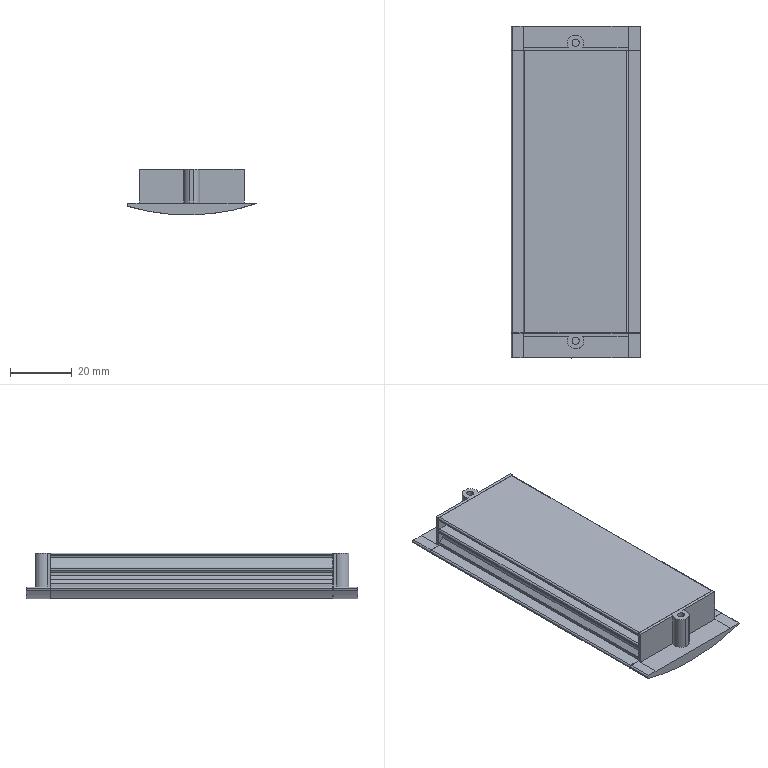Part | SolidWorks | features BaseBody 3 | 3 solids | 101 faces | box 42.062 x 107.5 x 14.849 mm | volume 13665 mm3 | plane 53 | cylinder 48 | commonest cylinder face diameters 1 x18 5.3 x6 139.273 x5 0.2 x4 2.3 x4 2.6 x3